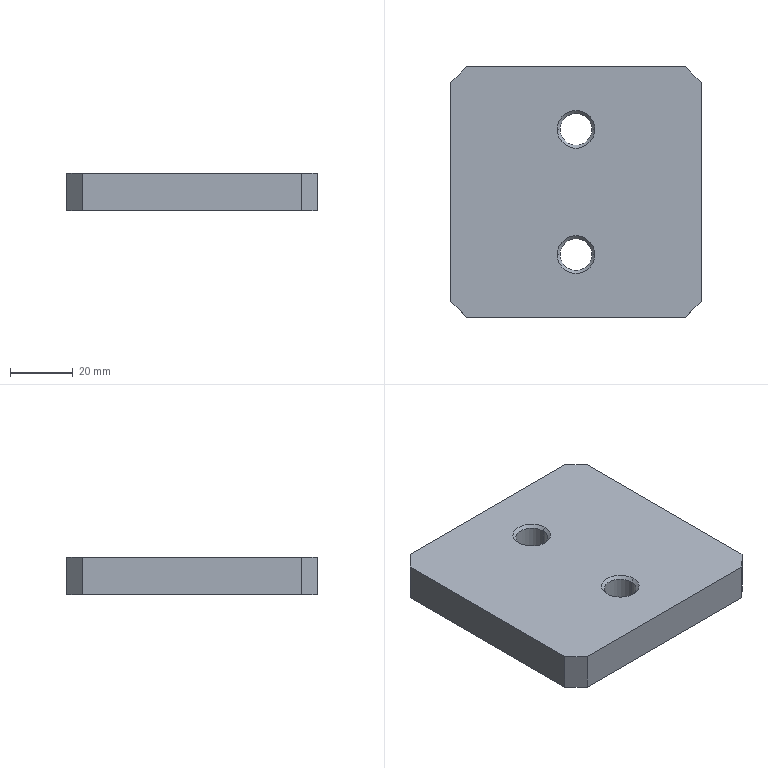Part | SolidWorks | features 3DProfileFeature 1, Chamfer 1, Extrusion 1, HoleWzd 1 | 1 solid | 18 faces | box 80 x 80 x 12 mm | volume 74210 mm3 | plane 10 | cone 4 | cylinder 4 | commonest cylinder face diameters 10.2 x4
STEP:
#1=CARTESIAN_POINT('',(-5.1,20.,11.075));
#2=VERTEX_POINT('',#1);
#3=CARTESIAN_POINT('',(5.1,20.,11.075));
#4=VERTEX_POINT('',#3);
#5=CARTESIAN_POINT('',(0.,20.,11.075));
#6=DIRECTION('',(0.,0.,1.));
#7=DIRECTION('',(1.,0.,0.));
#8=AXIS2_PLACEMENT_3D('',#5,#6,#7);
#9=CIRCLE('',#8,5.1);
#10=EDGE_CURVE('',#2,#4,#9,.T.);
#11=ORIENTED_EDGE('',*,*,#10,.F.);
#12=CARTESIAN_POINT('',(-6.025,20.,12.));
#13=VERTEX_POINT('',#12);
#14=CARTESIAN_POINT('',(-6.025,20.,12.));
#15=DIRECTION('',(-0.7071,0.,0.7071));
#16=VECTOR('',#15,1000.);
#17=LINE('',#14,#16);
#18=EDGE_CURVE('',#2,#13,#17,.T.);
#19=ORIENTED_EDGE('',*,*,#18,.T.);
#20=CARTESIAN_POINT('',(6.025,20.,12.));
#21=VERTEX_POINT('',#20);
#22=CARTESIAN_POINT('',(0.,20.,12.));
#23=DIRECTION('',(0.,0.,1.));
#24=DIRECTION('',(1.,0.,0.));
#25=AXIS2_PLACEMENT_3D('',#22,#23,#24);
#26=CIRCLE('',#25,6.025);
#27=EDGE_CURVE('',#13,#21,#26,.T.);
#28=ORIENTED_EDGE('',*,*,#27,.T.);
#29=CARTESIAN_POINT('',(6.025,20.,12.));
#30=DIRECTION('',(0.7071,0.,0.7071));
#31=VECTOR('',#30,1000.);
#32=LINE('',#29,#31);
#33=EDGE_CURVE('',#4,#21,#32,.T.);
#34=ORIENTED_EDGE('',*,*,#33,.F.);
#35=EDGE_LOOP('',(#11,#19,#28,#34));
#36=FACE_OUTER_BOUND('',#35,.T.);
#37=CARTESIAN_POINT('',(0.,20.,12.));
#38=DIRECTION('',(0.,0.,1.));
#39=DIRECTION('',(1.,0.,0.));
#40=AXIS2_PLACEMENT_3D('',#37,#38,#39);
#41=CONICAL_SURFACE('',#40,6.025,0.7854);
#42=ADVANCED_FACE('',(#36),#41,.F.);
#43=CARTESIAN_POINT('',(-5.1,20.,0.));
#44=VERTEX_POINT('',#43);
#45=CARTESIAN_POINT('',(5.1,20.,0.));
#46=VERTEX_POINT('',#45);
#47=CARTESIAN_POINT('',(0.,20.,0.));
#48=DIRECTION('',(0.,0.,1.));
#49=DIRECTION('',(1.,0.,0.));
#50=AXIS2_PLACEMENT_3D('',#47,#48,#49);
#51=CIRCLE('',#50,5.1);
#52=EDGE_CURVE('',#44,#46,#51,.T.);
#53=ORIENTED_EDGE('',*,*,#52,.F.);
#54=CARTESIAN_POINT('',(-5.1,20.,12.));
#55=DIRECTION('',(0.,0.,1.));
#56=VECTOR('',#55,1000.);
#57=LINE('',#54,#56);
#58=EDGE_CURVE('',#44,#2,#57,.T.);
#59=ORIENTED_EDGE('',*,*,#58,.T.);
#60=ORIENTED_EDGE('',*,*,#10,.T.);
#61=CARTESIAN_POINT('',(5.1,20.,12.));
#62=DIRECTION('',(0.,0.,1.));
#63=VECTOR('',#62,1000.);
#64=LINE('',#61,#63);
#65=EDGE_CURVE('',#46,#4,#64,.T.);
#66=ORIENTED_EDGE('',*,*,#65,.F.);
#67=EDGE_LOOP('',(#53,#59,#60,#66));
#68=FACE_OUTER_BOUND('',#67,.T.);
#69=CARTESIAN_POINT('',(0.,20.,12.));
#70=DIRECTION('',(0.,0.,1.));
#71=DIRECTION('',(1.,0.,0.));
#72=AXIS2_PLACEMENT_3D('',#69,#70,#71);
#73=CYLINDRICAL_SURFACE('',#72,5.1);
#74=ADVANCED_FACE('',(#68),#73,.F.);
#75=CARTESIAN_POINT('',(-5.1,-20.,11.075));
#76=VERTEX_POINT('',#75);
#77=CARTESIAN_POINT('',(5.1,-20.,11.075));
#78=VERTEX_POINT('',#77);
#79=CARTESIAN_POINT('',(0.,-20.,11.075));
#80=DIRECTION('',(0.,0.,1.));
#81=DIRECTION('',(1.,0.,0.));
#82=AXIS2_PLACEMENT_3D('',#79,#80,#81);
#83=CIRCLE('',#82,5.1);
#84=EDGE_CURVE('',#76,#78,#83,.T.);
#85=ORIENTED_EDGE('',*,*,#84,.F.);
#86=CARTESIAN_POINT('',(-6.025,-20.,12.));
#87=VERTEX_POINT('',#86);
#88=CARTESIAN_POINT('',(-6.025,-20.,12.));
#89=DIRECTION('',(-0.7071,0.,0.7071));
#90=VECTOR('',#89,1000.);
#91=LINE('',#88,#90);
#92=EDGE_CURVE('',#76,#87,#91,.T.);
#93=ORIENTED_EDGE('',*,*,#92,.T.);
#94=CARTESIAN_POINT('',(6.025,-20.,12.));
#95=VERTEX_POINT('',#94);
#96=CARTESIAN_POINT('',(0.,-20.,12.));
#97=DIRECTION('',(0.,0.,1.));
#98=DIRECTION('',(1.,0.,0.));
#99=AXIS2_PLACEMENT_3D('',#96,#97,#98);
#100=CIRCLE('',#99,6.025);
#101=EDGE_CURVE('',#87,#95,#100,.T.);
#102=ORIENTED_EDGE('',*,*,#101,.T.);
#103=CARTESIAN_POINT('',(6.025,-20.,12.));
#104=DIRECTION('',(0.7071,0.,0.7071));
#105=VECTOR('',#104,1000.);
#106=LINE('',#103,#105);
#107=EDGE_CURVE('',#78,#95,#106,.T.);
#108=ORIENTED_EDGE('',*,*,#107,.F.);
#109=EDGE_LOOP('',(#85,#93,#102,#108));
#110=FACE_OUTER_BOUND('',#109,.T.);
#111=CARTESIAN_POINT('',(0.,-20.,12.));
#112=DIRECTION('',(0.,0.,1.));
#113=DIRECTION('',(1.,0.,0.));
#114=AXIS2_PLACEMENT_3D('',#111,#112,#113);
#115=CONICAL_SURFACE('',#114,6.025,0.7854);
#116=ADVANCED_FACE('',(#110),#115,.F.);
#117=CARTESIAN_POINT('',(-5.1,-20.,0.));
#118=VERTEX_POINT('',#117);
#119=CARTESIAN_POINT('',(5.1,-20.,0.));
#120=VERTEX_POINT('',#119);
#121=CARTESIAN_POINT('',(0.,-20.,0.));
#122=DIRECTION('',(0.,0.,1.));
#123=DIRECTION('',(1.,0.,0.));
#124=AXIS2_PLACEMENT_3D('',#121,#122,#123);
#125=CIRCLE('',#124,5.1);
#126=EDGE_CURVE('',#118,#120,#125,.T.);
#127=ORIENTED_EDGE('',*,*,#126,.F.);
#128=CARTESIAN_POINT('',(-5.1,-20.,12.));
#129=DIRECTION('',(0.,0.,1.));
#130=VECTOR('',#129,1000.);
#131=LINE('',#128,#130);
#132=EDGE_CURVE('',#118,#76,#131,.T.);
#133=ORIENTED_EDGE('',*,*,#132,.T.);
#134=ORIENTED_EDGE('',*,*,#84,.T.);
#135=CARTESIAN_POINT('',(5.1,-20.,12.));
#136=DIRECTION('',(0.,0.,1.));
#137=VECTOR('',#136,1000.);
#138=LINE('',#135,#137);
#139=EDGE_CURVE('',#120,#78,#138,.T.);
#140=ORIENTED_EDGE('',*,*,#139,.F.);
#141=EDGE_LOOP('',(#127,#133,#134,#140));
#142=FACE_OUTER_BOUND('',#141,.T.);
#143=CARTESIAN_POINT('',(0.,-20.,12.));
#144=DIRECTION('',(0.,0.,1.));
#145=DIRECTION('',(1.,0.,0.));
#146=AXIS2_PLACEMENT_3D('',#143,#144,#145);
#147=CYLINDRICAL_SURFACE('',#146,5.1);
#148=ADVANCED_FACE('',(#142),#147,.F.);
#149=CARTESIAN_POINT('',(40.,-35.,12.));
#150=VERTEX_POINT('',#149);
#151=CARTESIAN_POINT('',(40.,35.,12.));
#152=VERTEX_POINT('',#151);
#153=CARTESIAN_POINT('',(40.,40.,12.));
#154=DIRECTION('',(0.,1.,0.));
#155=VECTOR('',#154,1000.);
#156=LINE('',#153,#155);
#157=EDGE_CURVE('',#150,#152,#156,.T.);
#158=ORIENTED_EDGE('',*,*,#157,.F.);
#159=CARTESIAN_POINT('',(40.,-35.,0.));
#160=VERTEX_POINT('',#159);
#161=CARTESIAN_POINT('',(40.,-35.,12.));
#162=DIRECTION('',(0.,0.,-1.));
#163=VECTOR('',#162,1000.);
#164=LINE('',#161,#163);
#165=EDGE_CURVE('',#150,#160,#164,.T.);
#166=ORIENTED_EDGE('',*,*,#165,.T.);
#167=CARTESIAN_POINT('',(40.,35.,0.));
#168=VERTEX_POINT('',#167);
#169=CARTESIAN_POINT('',(40.,40.,0.));
#170=DIRECTION('',(0.,1.,0.));
#171=VECTOR('',#170,1000.);
#172=LINE('',#169,#171);
#173=EDGE_CURVE('',#160,#168,#172,.T.);
#174=ORIENTED_EDGE('',*,*,#173,.T.);
#175=CARTESIAN_POINT('',(40.,35.,12.));
#176=DIRECTION('',(0.,0.,1.));
#177=VECTOR('',#176,1000.);
#178=LINE('',#175,#177);
#179=EDGE_CURVE('',#168,#152,#178,.T.);
#180=ORIENTED_EDGE('',*,*,#179,.T.);
#181=EDGE_LOOP('',(#158,#166,#174,#180));
#182=FACE_OUTER_BOUND('',#181,.T.);
#183=CARTESIAN_POINT('',(40.,40.,12.));
#184=DIRECTION('',(-1.,0.,0.));
#185=DIRECTION('',(0.,-1.,0.));
#186=AXIS2_PLACEMENT_3D('',#183,#184,#185);
#187=PLANE('',#186);
#188=ADVANCED_FACE('',(#182),#187,.F.);
#189=CARTESIAN_POINT('',(35.,40.,12.));
#190=VERTEX_POINT('',#189);
#191=CARTESIAN_POINT('',(-35.,40.,12.));
#192=VERTEX_POINT('',#191);
#193=CARTESIAN_POINT('',(-40.,40.,12.));
#194=DIRECTION('',(-1.,0.,0.));
#195=VECTOR('',#194,1000.);
#196=LINE('',#193,#195);
#197=EDGE_CURVE('',#190,#192,#196,.T.);
#198=ORIENTED_EDGE('',*,*,#197,.F.);
#199=CARTESIAN_POINT('',(35.,40.,0.));
#200=VERTEX_POINT('',#199);
#201=CARTESIAN_POINT('',(35.,40.,12.));
#202=DIRECTION('',(0.,0.,-1.));
#203=VECTOR('',#202,1000.);
#204=LINE('',#201,#203);
#205=EDGE_CURVE('',#190,#200,#204,.T.);
#206=ORIENTED_EDGE('',*,*,#205,.T.);
#207=CARTESIAN_POINT('',(-35.,40.,0.));
#208=VERTEX_POINT('',#207);
#209=CARTESIAN_POINT('',(-40.,40.,0.));
#210=DIRECTION('',(-1.,0.,0.));
#211=VECTOR('',#210,1000.);
#212=LINE('',#209,#211);
#213=EDGE_CURVE('',#200,#208,#212,.T.);
#214=ORIENTED_EDGE('',*,*,#213,.T.);
#215=CARTESIAN_POINT('',(-35.,40.,12.));
#216=DIRECTION('',(0.,0.,1.));
#217=VECTOR('',#216,1000.);
#218=LINE('',#215,#217);
#219=EDGE_CURVE('',#208,#192,#218,.T.);
#220=ORIENTED_EDGE('',*,*,#219,.T.);
#221=EDGE_LOOP('',(#198,#206,#214,#220));
#222=FACE_OUTER_BOUND('',#221,.T.);
#223=CARTESIAN_POINT('',(-40.,40.,12.));
#224=DIRECTION('',(0.,-1.,0.));
#225=DIRECTION('',(0.,0.,-1.));
#226=AXIS2_PLACEMENT_3D('',#223,#224,#225);
#227=PLANE('',#226);
#228=ADVANCED_FACE('',(#222),#227,.F.);
#229=CARTESIAN_POINT('',(-40.,35.,0.));
#230=VERTEX_POINT('',#229);
#231=CARTESIAN_POINT('',(-40.,-35.,0.));
#232=VERTEX_POINT('',#231);
#233=CARTESIAN_POINT('',(-40.,40.,0.));
#234=DIRECTION('',(0.,-1.,0.));
#235=VECTOR('',#234,1000.);
#236=LINE('',#233,#235);
#237=EDGE_CURVE('',#230,#232,#236,.T.);
#238=ORIENTED_EDGE('',*,*,#237,.T.);
#239=CARTESIAN_POINT('',(-40.,-35.,12.));
#240=VERTEX_POINT('',#239);
#241=CARTESIAN_POINT('',(-40.,-35.,12.));
#242=DIRECTION('',(0.,0.,1.));
#243=VECTOR('',#242,1000.);
#244=LINE('',#241,#243);
#245=EDGE_CURVE('',#232,#240,#244,.T.);
#246=ORIENTED_EDGE('',*,*,#245,.T.);
#247=CARTESIAN_POINT('',(-40.,35.,12.));
#248=VERTEX_POINT('',#247);
#249=CARTESIAN_POINT('',(-40.,40.,12.));
#250=DIRECTION('',(0.,-1.,0.));
#251=VECTOR('',#250,1000.);
#252=LINE('',#249,#251);
#253=EDGE_CURVE('',#248,#240,#252,.T.);
#254=ORIENTED_EDGE('',*,*,#253,.F.);
#255=CARTESIAN_POINT('',(-40.,35.,12.));
#256=DIRECTION('',(0.,0.,-1.));
#257=VECTOR('',#256,1000.);
#258=LINE('',#255,#257);
#259=EDGE_CURVE('',#248,#230,#258,.T.);
#260=ORIENTED_EDGE('',*,*,#259,.T.);
#261=EDGE_LOOP('',(#238,#246,#254,#260));
#262=FACE_OUTER_BOUND('',#261,.T.);
#263=CARTESIAN_POINT('',(-40.,40.,12.));
#264=DIRECTION('',(1.,0.,0.));
#265=DIRECTION('',(0.,1.,0.));
#266=AXIS2_PLACEMENT_3D('',#263,#264,#265);
#267=PLANE('',#266);
#268=ADVANCED_FACE('',(#262),#267,.F.);
#269=CARTESIAN_POINT('',(-35.,-40.,0.));
#270=VERTEX_POINT('',#269);
#271=CARTESIAN_POINT('',(35.,-40.,0.));
#272=VERTEX_POINT('',#271);
#273=CARTESIAN_POINT('',(-40.,-40.,0.));
#274=DIRECTION('',(1.,0.,0.));
#275=VECTOR('',#274,1000.);
#276=LINE('',#273,#275);
#277=EDGE_CURVE('',#270,#272,#276,.T.);
#278=ORIENTED_EDGE('',*,*,#277,.T.);
#279=CARTESIAN_POINT('',(35.,-40.,12.));
#280=VERTEX_POINT('',#279);
#281=CARTESIAN_POINT('',(35.,-40.,12.));
#282=DIRECTION('',(0.,0.,1.));
#283=VECTOR('',#282,1000.);
#284=LINE('',#281,#283);
#285=EDGE_CURVE('',#272,#280,#284,.T.);
#286=ORIENTED_EDGE('',*,*,#285,.T.);
#287=CARTESIAN_POINT('',(-35.,-40.,12.));
#288=VERTEX_POINT('',#287);
#289=CARTESIAN_POINT('',(-40.,-40.,12.));
#290=DIRECTION('',(1.,0.,0.));
#291=VECTOR('',#290,1000.);
#292=LINE('',#289,#291);
#293=EDGE_CURVE('',#288,#280,#292,.T.);
#294=ORIENTED_EDGE('',*,*,#293,.F.);
#295=CARTESIAN_POINT('',(-35.,-40.,12.));
#296=DIRECTION('',(0.,0.,-1.));
#297=VECTOR('',#296,1000.);
#298=LINE('',#295,#297);
#299=EDGE_CURVE('',#288,#270,#298,.T.);
#300=ORIENTED_EDGE('',*,*,#299,.T.);
#301=EDGE_LOOP('',(#278,#286,#294,#300));
#302=FACE_OUTER_BOUND('',#301,.T.);
#303=CARTESIAN_POINT('',(-40.,-40.,12.));
#304=DIRECTION('',(0.,1.,0.));
#305=DIRECTION('',(0.,0.,1.));
#306=AXIS2_PLACEMENT_3D('',#303,#304,#305);
#307=PLANE('',#306);
#308=ADVANCED_FACE('',(#302),#307,.F.);
#309=CARTESIAN_POINT('',(0.,20.,12.));
#310=DIRECTION('',(0.,0.,1.));
#311=DIRECTION('',(1.,0.,0.));
#312=AXIS2_PLACEMENT_3D('',#309,#310,#311);
#313=CIRCLE('',#312,6.025);
#314=EDGE_CURVE('',#21,#13,#313,.T.);
#315=ORIENTED_EDGE('',*,*,#314,.F.);
#316=ORIENTED_EDGE('',*,*,#27,.F.);
#317=EDGE_LOOP('',(#315,#316));
#318=FACE_BOUND('',#317,.T.);
#319=CARTESIAN_POINT('',(0.,-20.,12.));
#320=DIRECTION('',(0.,0.,1.));
#321=DIRECTION('',(1.,0.,0.));
#322=AXIS2_PLACEMENT_3D('',#319,#320,#321);
#323=CIRCLE('',#322,6.025);
#324=EDGE_CURVE('',#95,#87,#323,.T.);
#325=ORIENTED_EDGE('',*,*,#324,.F.);
#326=ORIENTED_EDGE('',*,*,#101,.F.);
#327=EDGE_LOOP('',(#325,#326));
#328=FACE_BOUND('',#327,.T.);
#329=ORIENTED_EDGE('',*,*,#293,.T.);
#330=CARTESIAN_POINT('',(37.5,-37.5,12.));
#331=DIRECTION('',(0.7071,0.7071,0.));
#332=VECTOR('',#331,1000.);
#333=LINE('',#330,#332);
#334=EDGE_CURVE('',#280,#150,#333,.T.);
#335=ORIENTED_EDGE('',*,*,#334,.T.);
#336=ORIENTED_EDGE('',*,*,#157,.T.);
#337=CARTESIAN_POINT('',(37.5,37.5,12.));
#338=DIRECTION('',(-0.7071,0.7071,0.));
#339=VECTOR('',#338,1000.);
#340=LINE('',#337,#339);
#341=EDGE_CURVE('',#152,#190,#340,.T.);
#342=ORIENTED_EDGE('',*,*,#341,.T.);
#343=ORIENTED_EDGE('',*,*,#197,.T.);
#344=CARTESIAN_POINT('',(-37.5,37.5,12.));
#345=DIRECTION('',(-0.7071,-0.7071,0.));
#346=VECTOR('',#345,1000.);
#347=LINE('',#344,#346);
#348=EDGE_CURVE('',#192,#248,#347,.T.);
#349=ORIENTED_EDGE('',*,*,#348,.T.);
#350=ORIENTED_EDGE('',*,*,#253,.T.);
#351=CARTESIAN_POINT('',(-37.5,-37.5,12.));
#352=DIRECTION('',(0.7071,-0.7071,0.));
#353=VECTOR('',#352,1000.);
#354=LINE('',#351,#353);
#355=EDGE_CURVE('',#240,#288,#354,.T.);
#356=ORIENTED_EDGE('',*,*,#355,.T.);
#357=EDGE_LOOP('',(#329,#335,#336,#342,#343,#349,#350,#356));
#358=FACE_OUTER_BOUND('',#357,.T.);
#359=CARTESIAN_POINT('',(0.,0.,12.));
#360=DIRECTION('',(0.,0.,1.));
#361=DIRECTION('',(1.,0.,0.));
#362=AXIS2_PLACEMENT_3D('',#359,#360,#361);
#363=PLANE('',#362);
#364=ADVANCED_FACE('',(#318,#328,#358),#363,.T.);
#365=CARTESIAN_POINT('',(0.,20.,0.));
#366=DIRECTION('',(0.,0.,1.));
#367=DIRECTION('',(1.,0.,0.));
#368=AXIS2_PLACEMENT_3D('',#365,#366,#367);
#369=CIRCLE('',#368,5.1);
#370=EDGE_CURVE('',#46,#44,#369,.T.);
#371=ORIENTED_EDGE('',*,*,#370,.T.);
#372=ORIENTED_EDGE('',*,*,#52,.T.);
#373=EDGE_LOOP('',(#371,#372));
#374=FACE_BOUND('',#373,.T.);
#375=CARTESIAN_POINT('',(0.,-20.,0.));
#376=DIRECTION('',(0.,0.,1.));
#377=DIRECTION('',(1.,0.,0.));
#378=AXIS2_PLACEMENT_3D('',#375,#376,#377);
#379=CIRCLE('',#378,5.1);
#380=EDGE_CURVE('',#120,#118,#379,.T.);
#381=ORIENTED_EDGE('',*,*,#380,.T.);
#382=ORIENTED_EDGE('',*,*,#126,.T.);
#383=EDGE_LOOP('',(#381,#382));
#384=FACE_BOUND('',#383,.T.);
#385=ORIENTED_EDGE('',*,*,#173,.F.);
#386=CARTESIAN_POINT('',(40.,-35.,0.));
#387=DIRECTION('',(-0.7071,-0.7071,0.));
#388=VECTOR('',#387,1000.);
#389=LINE('',#386,#388);
#390=EDGE_CURVE('',#160,#272,#389,.T.);
#391=ORIENTED_EDGE('',*,*,#390,.T.);
#392=ORIENTED_EDGE('',*,*,#277,.F.);
#393=CARTESIAN_POINT('',(-35.,-40.,0.));
#394=DIRECTION('',(-0.7071,0.7071,0.));
#395=VECTOR('',#394,1000.);
#396=LINE('',#393,#395);
#397=EDGE_CURVE('',#270,#232,#396,.T.);
#398=ORIENTED_EDGE('',*,*,#397,.T.);
#399=ORIENTED_EDGE('',*,*,#237,.F.);
#400=CARTESIAN_POINT('',(-40.,35.,0.));
#401=DIRECTION('',(0.7071,0.7071,0.));
#402=VECTOR('',#401,1000.);
#403=LINE('',#400,#402);
#404=EDGE_CURVE('',#230,#208,#403,.T.);
#405=ORIENTED_EDGE('',*,*,#404,.T.);
#406=ORIENTED_EDGE('',*,*,#213,.F.);
#407=CARTESIAN_POINT('',(35.,40.,0.));
#408=DIRECTION('',(0.7071,-0.7071,0.));
#409=VECTOR('',#408,1000.);
#410=LINE('',#407,#409);
#411=EDGE_CURVE('',#200,#168,#410,.T.);
#412=ORIENTED_EDGE('',*,*,#411,.T.);
#413=EDGE_LOOP('',(#385,#391,#392,#398,#399,#405,#406,#412));
#414=FACE_OUTER_BOUND('',#413,.T.);
#415=CARTESIAN_POINT('',(0.,0.,0.));
#416=DIRECTION('',(0.,0.,1.));
#417=DIRECTION('',(1.,0.,0.));
#418=AXIS2_PLACEMENT_3D('',#415,#416,#417);
#419=PLANE('',#418);
#420=ADVANCED_FACE('',(#374,#384,#414),#419,.F.);
#421=ORIENTED_EDGE('',*,*,#334,.F.);
#422=ORIENTED_EDGE('',*,*,#285,.F.);
#423=ORIENTED_EDGE('',*,*,#390,.F.);
#424=ORIENTED_EDGE('',*,*,#165,.F.);
#425=EDGE_LOOP('',(#421,#422,#423,#424));
#426=FACE_OUTER_BOUND('',#425,.T.);
#427=CARTESIAN_POINT('',(40.,-35.,12.));
#428=DIRECTION('',(-0.7071,0.7071,0.));
#429=DIRECTION('',(0.,0.,-1.));
#430=AXIS2_PLACEMENT_3D('',#427,#428,#429);
#431=PLANE('',#430);
#432=ADVANCED_FACE('',(#426),#431,.F.);
#433=ORIENTED_EDGE('',*,*,#355,.F.);
#434=ORIENTED_EDGE('',*,*,#245,.F.);
#435=ORIENTED_EDGE('',*,*,#397,.F.);
#436=ORIENTED_EDGE('',*,*,#299,.F.);
#437=EDGE_LOOP('',(#433,#434,#435,#436));
#438=FACE_OUTER_BOUND('',#437,.T.);
#439=CARTESIAN_POINT('',(-35.,-40.,12.));
#440=DIRECTION('',(0.7071,0.7071,0.));
#441=DIRECTION('',(0.,0.,-1.));
#442=AXIS2_PLACEMENT_3D('',#439,#440,#441);
#443=PLANE('',#442);
#444=ADVANCED_FACE('',(#438),#443,.F.);
#445=ORIENTED_EDGE('',*,*,#341,.F.);
#446=ORIENTED_EDGE('',*,*,#179,.F.);
#447=ORIENTED_EDGE('',*,*,#411,.F.);
#448=ORIENTED_EDGE('',*,*,#205,.F.);
#449=EDGE_LOOP('',(#445,#446,#447,#448));
#450=FACE_OUTER_BOUND('',#449,.T.);
#451=CARTESIAN_POINT('',(35.,40.,12.));
#452=DIRECTION('',(-0.7071,-0.7071,0.));
#453=DIRECTION('',(0.,0.,-1.));
#454=AXIS2_PLACEMENT_3D('',#451,#452,#453);
#455=PLANE('',#454);
#456=ADVANCED_FACE('',(#450),#455,.F.);
#457=ORIENTED_EDGE('',*,*,#348,.F.);
#458=ORIENTED_EDGE('',*,*,#219,.F.);
#459=ORIENTED_EDGE('',*,*,#404,.F.);
#460=ORIENTED_EDGE('',*,*,#259,.F.);
#461=EDGE_LOOP('',(#457,#458,#459,#460));
#462=FACE_OUTER_BOUND('',#461,.T.);
#463=CARTESIAN_POINT('',(-40.,35.,12.));
#464=DIRECTION('',(0.7071,-0.7071,0.));
#465=DIRECTION('',(0.,0.,-1.));
#466=AXIS2_PLACEMENT_3D('',#463,#464,#465);
#467=PLANE('',#466);
#468=ADVANCED_FACE('',(#462),#467,.F.);
#469=ORIENTED_EDGE('',*,*,#132,.F.);
#470=ORIENTED_EDGE('',*,*,#380,.F.);
#471=ORIENTED_EDGE('',*,*,#139,.T.);
#472=CARTESIAN_POINT('',(0.,-20.,11.075));
#473=DIRECTION('',(0.,0.,1.));
#474=DIRECTION('',(1.,0.,0.));
#475=AXIS2_PLACEMENT_3D('',#472,#473,#474);
#476=CIRCLE('',#475,5.1);
#477=EDGE_CURVE('',#78,#76,#476,.T.);
#478=ORIENTED_EDGE('',*,*,#477,.T.);
#479=EDGE_LOOP('',(#469,#470,#471,#478));
#480=FACE_OUTER_BOUND('',#479,.T.);
#481=CARTESIAN_POINT('',(0.,-20.,12.));
#482=DIRECTION('',(0.,0.,1.));
#483=DIRECTION('',(1.,0.,0.));
#484=AXIS2_PLACEMENT_3D('',#481,#482,#483);
#485=CYLINDRICAL_SURFACE('',#484,5.1);
#486=ADVANCED_FACE('',(#480),#485,.F.);
#487=ORIENTED_EDGE('',*,*,#92,.F.);
#488=ORIENTED_EDGE('',*,*,#477,.F.);
#489=ORIENTED_EDGE('',*,*,#107,.T.);
#490=ORIENTED_EDGE('',*,*,#324,.T.);
#491=EDGE_LOOP('',(#487,#488,#489,#490));
#492=FACE_OUTER_BOUND('',#491,.T.);
#493=CARTESIAN_POINT('',(0.,-20.,12.));
#494=DIRECTION('',(0.,0.,1.));
#495=DIRECTION('',(1.,0.,0.));
#496=AXIS2_PLACEMENT_3D('',#493,#494,#495);
#497=CONICAL_SURFACE('',#496,6.025,0.7854);
#498=ADVANCED_FACE('',(#492),#497,.F.);
#499=ORIENTED_EDGE('',*,*,#58,.F.);
#500=ORIENTED_EDGE('',*,*,#370,.F.);
#501=ORIENTED_EDGE('',*,*,#65,.T.);
#502=CARTESIAN_POINT('',(0.,20.,11.075));
#503=DIRECTION('',(0.,0.,1.));
#504=DIRECTION('',(1.,0.,0.));
#505=AXIS2_PLACEMENT_3D('',#502,#503,#504);
#506=CIRCLE('',#505,5.1);
#507=EDGE_CURVE('',#4,#2,#506,.T.);
#508=ORIENTED_EDGE('',*,*,#507,.T.);
#509=EDGE_LOOP('',(#499,#500,#501,#508));
#510=FACE_OUTER_BOUND('',#509,.T.);
#511=CARTESIAN_POINT('',(0.,20.,12.));
#512=DIRECTION('',(0.,0.,1.));
#513=DIRECTION('',(1.,0.,0.));
#514=AXIS2_PLACEMENT_3D('',#511,#512,#513);
#515=CYLINDRICAL_SURFACE('',#514,5.1);
#516=ADVANCED_FACE('',(#510),#515,.F.);
#517=ORIENTED_EDGE('',*,*,#18,.F.);
#518=ORIENTED_EDGE('',*,*,#507,.F.);
#519=ORIENTED_EDGE('',*,*,#33,.T.);
#520=ORIENTED_EDGE('',*,*,#314,.T.);
#521=EDGE_LOOP('',(#517,#518,#519,#520));
#522=FACE_OUTER_BOUND('',#521,.T.);
#523=CARTESIAN_POINT('',(0.,20.,12.));
#524=DIRECTION('',(0.,0.,1.));
#525=DIRECTION('',(1.,0.,0.));
#526=AXIS2_PLACEMENT_3D('',#523,#524,#525);
#527=CONICAL_SURFACE('',#526,6.025,0.7854);
#528=ADVANCED_FACE('',(#522),#527,.F.);
#529=CLOSED_SHELL('',(#42,#74,#116,#148,#188,#228,#268,#308,#364,#420,#432,#444,#456,#468,#486,#498,#516,#528));
#530=MANIFOLD_SOLID_BREP('',#529);
#531=CARTESIAN_POINT('',(0.,0.,0.));
#532=DIRECTION('',(0.,0.,1.));
#533=DIRECTION('',(1.,0.,0.));
#534=AXIS2_PLACEMENT_3D('',#531,#532,#533);
#535=(LENGTH_UNIT()NAMED_UNIT(*)SI_UNIT(.MILLI.,.METRE.));
#536=UNCERTAINTY_MEASURE_WITH_UNIT(LENGTH_MEASURE(0.00001),#535,'','');
#537=(NAMED_UNIT(*)PLANE_ANGLE_UNIT()SI_UNIT($,.RADIAN.));
#538=(NAMED_UNIT(*)SI_UNIT($,.STERADIAN.)SOLID_ANGLE_UNIT());
#539=(GEOMETRIC_REPRESENTATION_CONTEXT(3)GLOBAL_UNCERTAINTY_ASSIGNED_CONTEXT((#536))GLOBAL_UNIT_ASSIGNED_CONTEXT((#535,#537,#538))REPRESENTATION_CONTEXT('',''));
#540=ADVANCED_BREP_SHAPE_REPRESENTATION('',(#530,#534),#539);